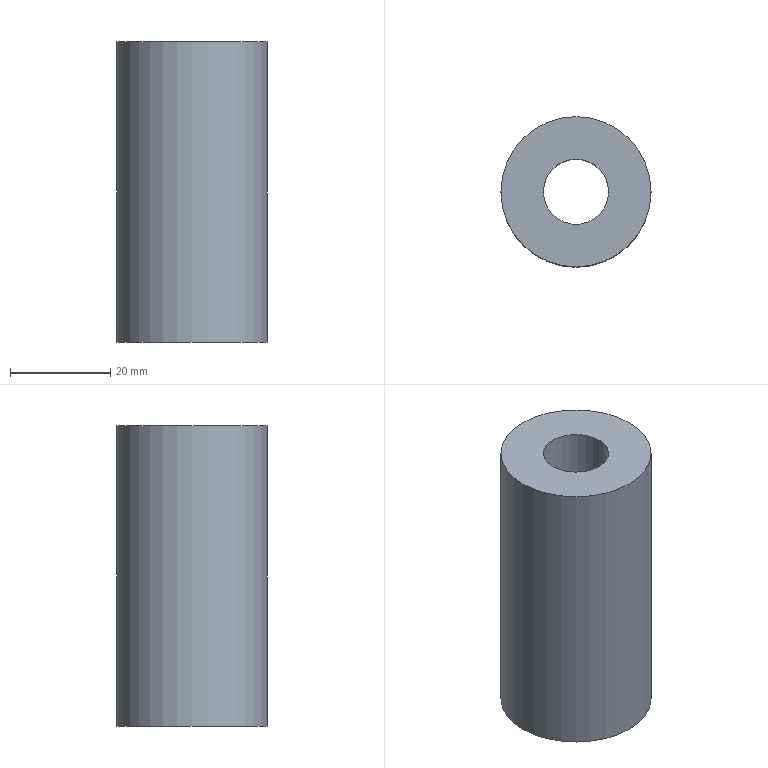Part | NX | features solid 2 | 1 solid | 6 faces | box 30 x 30 x 60 mm | volume 29005 mm3 | plane 3 | cylinder 3 | commonest cylinder face diameters 13 x1 20 x1 30 x1
STEP:
#1=CARTESIAN_POINT('',(621.5,115.,-29.));
#2=VERTEX_POINT('',#1);
#3=CARTESIAN_POINT('',(615.,115.,-29.));
#4=DIRECTION('',(-0.000000502,0.000000149,1.));
#5=DIRECTION('',(1.,0.,0.000000502));
#6=AXIS2_PLACEMENT_3D('',#3,#4,#5);
#7=CIRCLE('',#6,6.5);
#8=EDGE_CURVE('',#2,#2,#7,.T.);
#9=ORIENTED_EDGE('',*,*,#8,.F.);
#10=EDGE_LOOP('',(#9));
#11=FACE_BOUND('',#10,.T.);
#12=CARTESIAN_POINT('',(630.,115.,-29.));
#13=VERTEX_POINT('',#12);
#14=CARTESIAN_POINT('',(615.,115.,-29.));
#15=DIRECTION('',(-0.000000502,0.000000149,1.));
#16=DIRECTION('',(1.,0.,0.000000502));
#17=AXIS2_PLACEMENT_3D('',#14,#15,#16);
#18=CIRCLE('',#17,15.);
#19=EDGE_CURVE('',#13,#13,#18,.F.);
#20=ORIENTED_EDGE('',*,*,#19,.F.);
#21=EDGE_LOOP('',(#20));
#22=FACE_BOUND('',#21,.T.);
#23=CARTESIAN_POINT('',(615.,115.,-29.));
#24=DIRECTION('',(-0.000000502,0.000000149,1.));
#25=DIRECTION('',(1.,0.000001668,0.000000502));
#26=AXIS2_PLACEMENT_3D('',#23,#24,#25);
#27=PLANE('',#26);
#28=ADVANCED_FACE('',(#11,#22),#27,.T.);
#29=CARTESIAN_POINT('',(605.,115.,-89.));
#30=VERTEX_POINT('',#29);
#31=CARTESIAN_POINT('',(615.,115.,-89.));
#32=DIRECTION('',(0.000000502,-0.000000149,-1.));
#33=DIRECTION('',(-1.,0.,-0.000000502));
#34=AXIS2_PLACEMENT_3D('',#31,#32,#33);
#35=CIRCLE('',#34,10.);
#36=EDGE_CURVE('',#30,#30,#35,.F.);
#37=ORIENTED_EDGE('',*,*,#36,.T.);
#38=EDGE_LOOP('',(#37));
#39=FACE_BOUND('',#38,.T.);
#40=CARTESIAN_POINT('',(600.,115.,-89.));
#41=VERTEX_POINT('',#40);
#42=CARTESIAN_POINT('',(615.,115.,-89.));
#43=DIRECTION('',(0.000000502,-0.000000149,-1.));
#44=DIRECTION('',(-1.,0.,-0.000000502));
#45=AXIS2_PLACEMENT_3D('',#42,#43,#44);
#46=CIRCLE('',#45,15.);
#47=EDGE_CURVE('',#41,#41,#46,.F.);
#48=ORIENTED_EDGE('',*,*,#47,.F.);
#49=EDGE_LOOP('',(#48));
#50=FACE_BOUND('',#49,.T.);
#51=CARTESIAN_POINT('',(615.,115.,-89.));
#52=DIRECTION('',(0.000000502,-0.000000149,-1.));
#53=DIRECTION('',(-1.,-0.000001668,-0.000000502));
#54=AXIS2_PLACEMENT_3D('',#51,#52,#53);
#55=PLANE('',#54);
#56=ADVANCED_FACE('',(#39,#50),#55,.T.);
#57=ORIENTED_EDGE('',*,*,#19,.T.);
#58=EDGE_LOOP('',(#57));
#59=FACE_BOUND('',#58,.T.);
#60=ORIENTED_EDGE('',*,*,#47,.T.);
#61=EDGE_LOOP('',(#60));
#62=FACE_BOUND('',#61,.T.);
#63=CARTESIAN_POINT('',(615.,115.,-94.));
#64=DIRECTION('',(-0.000000502,0.000000149,1.));
#65=DIRECTION('',(1.,0.000001668,0.000000502));
#66=AXIS2_PLACEMENT_3D('',#63,#64,#65);
#67=CYLINDRICAL_SURFACE('',#66,15.);
#68=ADVANCED_FACE('',(#59,#62),#67,.T.);
#69=ORIENTED_EDGE('',*,*,#8,.T.);
#70=EDGE_LOOP('',(#69));
#71=FACE_BOUND('',#70,.T.);
#72=CARTESIAN_POINT('',(621.5,115.,-59.));
#73=VERTEX_POINT('',#72);
#74=CARTESIAN_POINT('',(615.,115.,-59.));
#75=DIRECTION('',(-0.000000502,0.000000149,1.));
#76=DIRECTION('',(1.,0.,0.000000502));
#77=AXIS2_PLACEMENT_3D('',#74,#75,#76);
#78=CIRCLE('',#77,6.5);
#79=EDGE_CURVE('',#73,#73,#78,.T.);
#80=ORIENTED_EDGE('',*,*,#79,.F.);
#81=EDGE_LOOP('',(#80));
#82=FACE_BOUND('',#81,.T.);
#83=CARTESIAN_POINT('',(615.,115.,21.));
#84=DIRECTION('',(-0.000000502,0.000000149,1.));
#85=DIRECTION('',(1.,0.000001668,0.000000502));
#86=AXIS2_PLACEMENT_3D('',#83,#84,#85);
#87=CYLINDRICAL_SURFACE('',#86,6.5);
#88=ADVANCED_FACE('',(#71,#82),#87,.F.);
#89=ORIENTED_EDGE('',*,*,#79,.T.);
#90=EDGE_LOOP('',(#89));
#91=FACE_BOUND('',#90,.T.);
#92=CARTESIAN_POINT('',(625.,115.,-59.));
#93=VERTEX_POINT('',#92);
#94=CARTESIAN_POINT('',(615.,115.,-59.));
#95=DIRECTION('',(-0.000000502,0.000000149,1.));
#96=DIRECTION('',(1.,0.,0.000000502));
#97=AXIS2_PLACEMENT_3D('',#94,#95,#96);
#98=CIRCLE('',#97,10.);
#99=EDGE_CURVE('',#93,#93,#98,.T.);
#100=ORIENTED_EDGE('',*,*,#99,.F.);
#101=EDGE_LOOP('',(#100));
#102=FACE_BOUND('',#101,.T.);
#103=CARTESIAN_POINT('',(615.,115.,-59.));
#104=DIRECTION('',(-0.000000502,0.000000149,1.));
#105=DIRECTION('',(1.,0.000001668,0.000000502));
#106=AXIS2_PLACEMENT_3D('',#103,#104,#105);
#107=PLANE('',#106);
#108=ADVANCED_FACE('',(#91,#102),#107,.F.);
#109=ORIENTED_EDGE('',*,*,#99,.T.);
#110=EDGE_LOOP('',(#109));
#111=FACE_BOUND('',#110,.T.);
#112=ORIENTED_EDGE('',*,*,#36,.F.);
#113=EDGE_LOOP('',(#112));
#114=FACE_BOUND('',#113,.T.);
#115=CARTESIAN_POINT('',(615.,115.,-79.));
#116=DIRECTION('',(-0.000000502,0.000000149,1.));
#117=DIRECTION('',(1.,0.000001668,0.000000502));
#118=AXIS2_PLACEMENT_3D('',#115,#116,#117);
#119=CYLINDRICAL_SURFACE('',#118,10.);
#120=ADVANCED_FACE('',(#111,#114),#119,.F.);
#121=CLOSED_SHELL('',(#28,#56,#68,#88,#108,#120));
#122=MANIFOLD_SOLID_BREP('',#121);
#123=(LENGTH_UNIT()NAMED_UNIT(*)SI_UNIT(.MILLI.,.METRE.));
#124=UNCERTAINTY_MEASURE_WITH_UNIT(LENGTH_MEASURE(0.00001),#123,'','');
#125=(NAMED_UNIT(*)PLANE_ANGLE_UNIT()SI_UNIT($,.RADIAN.));
#126=(NAMED_UNIT(*)SI_UNIT($,.STERADIAN.)SOLID_ANGLE_UNIT());
#127=(GEOMETRIC_REPRESENTATION_CONTEXT(3)GLOBAL_UNCERTAINTY_ASSIGNED_CONTEXT((#124))GLOBAL_UNIT_ASSIGNED_CONTEXT((#123,#125,#126))REPRESENTATION_CONTEXT('',''));
#128=ADVANCED_BREP_SHAPE_REPRESENTATION('',(#122),#127);